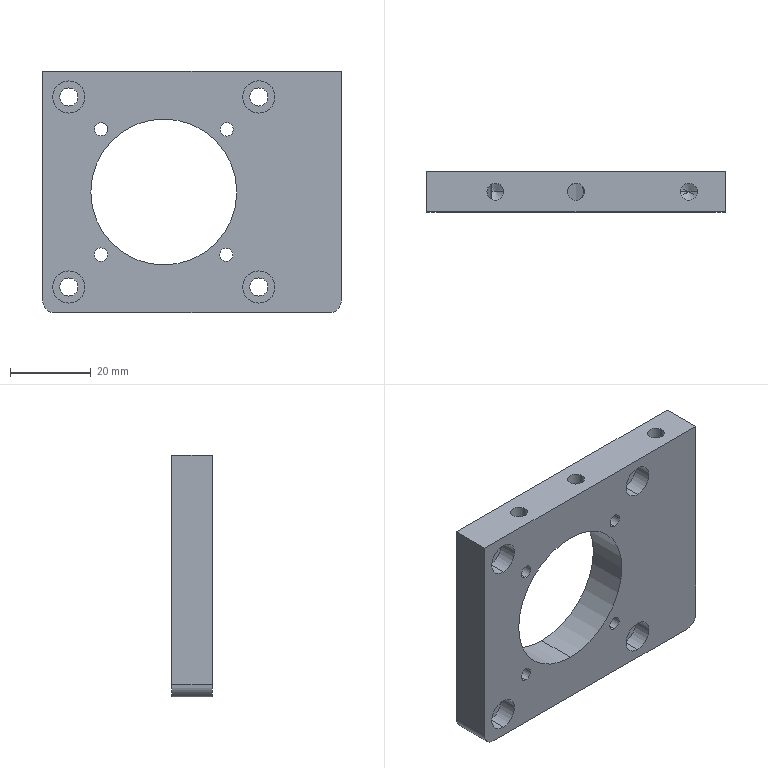Part | STEP file | PN_0008 | 1 solid | 62 faces | box 74 x 10 x 60 mm | volume 31735 mm3 | cylinder 42 | plane 14 | cone 6 | commonest cylinder face diameters 3.3 x8 4.5 x8 8 x8 8.1 x8 4.2 x6 6 x2